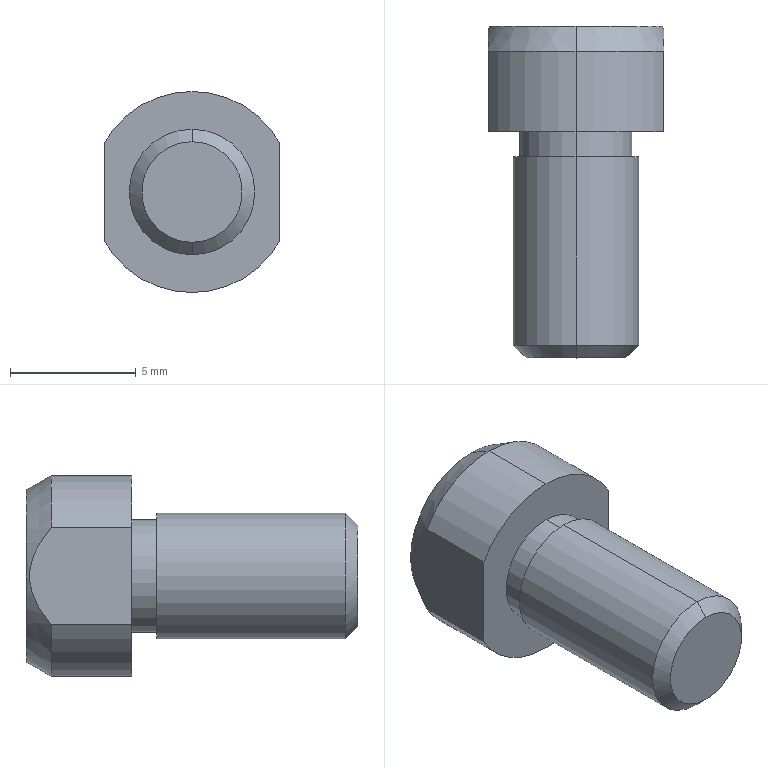Part | STEP file | PN_0011 Default | 1 solid | 17 faces | box 7 x 13.2 x 8 mm | volume 366.094 mm3 | cylinder 7 | plane 6 | cone 4 | commonest cylinder face diameters 8 x3 4.5 x2 5 x2
STEP:
#1=CARTESIAN_POINT('',(0.,14.722,-2.));
#2=VERTEX_POINT('',#1);
#3=CARTESIAN_POINT('',(0.,14.722,2.));
#4=VERTEX_POINT('',#3);
#5=CARTESIAN_POINT('',(0.,14.722,0.));
#6=DIRECTION('',(0.,-1.,0.));
#7=DIRECTION('',(0.,0.,-1.));
#8=AXIS2_PLACEMENT_3D('',#5,#6,#7);
#9=CIRCLE('',#8,2.);
#10=EDGE_CURVE('',#2,#4,#9,.T.);
#11=ORIENTED_EDGE('',*,*,#10,.F.);
#12=CARTESIAN_POINT('',(0.,15.222,-2.5));
#13=VERTEX_POINT('',#12);
#14=CARTESIAN_POINT('',(0.,15.222,-2.5));
#15=DIRECTION('',(0.,0.7071,-0.7071));
#16=VECTOR('',#15,1000.);
#17=LINE('',#14,#16);
#18=EDGE_CURVE('',#2,#13,#17,.T.);
#19=ORIENTED_EDGE('',*,*,#18,.T.);
#20=CARTESIAN_POINT('',(0.,15.222,2.5));
#21=VERTEX_POINT('',#20);
#22=CARTESIAN_POINT('',(0.,15.222,0.));
#23=DIRECTION('',(0.,1.,0.));
#24=DIRECTION('',(0.,0.,-1.));
#25=AXIS2_PLACEMENT_3D('',#22,#23,#24);
#26=CIRCLE('',#25,2.5);
#27=EDGE_CURVE('',#21,#13,#26,.T.);
#28=ORIENTED_EDGE('',*,*,#27,.F.);
#29=CARTESIAN_POINT('',(0.,15.222,2.5));
#30=DIRECTION('',(0.,0.7071,0.7071));
#31=VECTOR('',#30,1000.);
#32=LINE('',#29,#31);
#33=EDGE_CURVE('',#4,#21,#32,.T.);
#34=ORIENTED_EDGE('',*,*,#33,.F.);
#35=EDGE_LOOP('',(#11,#19,#28,#34));
#36=FACE_OUTER_BOUND('',#35,.T.);
#37=CARTESIAN_POINT('',(0.,15.222,0.));
#38=DIRECTION('',(0.,1.,0.));
#39=DIRECTION('',(0.,0.,1.));
#40=AXIS2_PLACEMENT_3D('',#37,#38,#39);
#41=CONICAL_SURFACE('',#40,2.5,0.7854);
#42=ADVANCED_FACE('',(#36),#41,.T.);
#43=ORIENTED_EDGE('',*,*,#27,.T.);
#44=CARTESIAN_POINT('',(0.,22.722,-2.5));
#45=VERTEX_POINT('',#44);
#46=CARTESIAN_POINT('',(0.,25.949,-2.5));
#47=DIRECTION('',(0.,1.,0.));
#48=VECTOR('',#47,1000.);
#49=LINE('',#46,#48);
#50=EDGE_CURVE('',#13,#45,#49,.T.);
#51=ORIENTED_EDGE('',*,*,#50,.T.);
#52=CARTESIAN_POINT('',(0.,22.722,2.5));
#53=VERTEX_POINT('',#52);
#54=CARTESIAN_POINT('',(0.,22.722,0.));
#55=DIRECTION('',(0.,1.,0.));
#56=DIRECTION('',(0.,0.,-1.));
#57=AXIS2_PLACEMENT_3D('',#54,#55,#56);
#58=CIRCLE('',#57,2.5);
#59=EDGE_CURVE('',#53,#45,#58,.T.);
#60=ORIENTED_EDGE('',*,*,#59,.F.);
#61=CARTESIAN_POINT('',(0.,25.949,2.5));
#62=DIRECTION('',(0.,1.,0.));
#63=VECTOR('',#62,1000.);
#64=LINE('',#61,#63);
#65=EDGE_CURVE('',#21,#53,#64,.T.);
#66=ORIENTED_EDGE('',*,*,#65,.F.);
#67=EDGE_LOOP('',(#43,#51,#60,#66));
#68=FACE_OUTER_BOUND('',#67,.T.);
#69=CARTESIAN_POINT('',(0.,25.949,0.));
#70=DIRECTION('',(0.,1.,0.));
#71=DIRECTION('',(0.,0.,1.));
#72=AXIS2_PLACEMENT_3D('',#69,#70,#71);
#73=CYLINDRICAL_SURFACE('',#72,2.5);
#74=ADVANCED_FACE('',(#68),#73,.T.);
#75=CARTESIAN_POINT('',(0.,22.722,-2.25));
#76=VERTEX_POINT('',#75);
#77=CARTESIAN_POINT('',(0.,22.722,2.25));
#78=VERTEX_POINT('',#77);
#79=CARTESIAN_POINT('',(0.,22.722,0.));
#80=DIRECTION('',(0.,-1.,0.));
#81=DIRECTION('',(0.,0.,-1.));
#82=AXIS2_PLACEMENT_3D('',#79,#80,#81);
#83=CIRCLE('',#82,2.25);
#84=EDGE_CURVE('',#76,#78,#83,.T.);
#85=ORIENTED_EDGE('',*,*,#84,.F.);
#86=CARTESIAN_POINT('',(0.,23.722,-2.25));
#87=VERTEX_POINT('',#86);
#88=CARTESIAN_POINT('',(0.,22.722,-2.25));
#89=DIRECTION('',(0.,1.,0.));
#90=VECTOR('',#89,1000.);
#91=LINE('',#88,#90);
#92=EDGE_CURVE('',#76,#87,#91,.T.);
#93=ORIENTED_EDGE('',*,*,#92,.T.);
#94=CARTESIAN_POINT('',(0.,23.722,2.25));
#95=VERTEX_POINT('',#94);
#96=CARTESIAN_POINT('',(0.,23.722,0.));
#97=DIRECTION('',(0.,-1.,0.));
#98=DIRECTION('',(0.,0.,-1.));
#99=AXIS2_PLACEMENT_3D('',#96,#97,#98);
#100=CIRCLE('',#99,2.25);
#101=EDGE_CURVE('',#87,#95,#100,.T.);
#102=ORIENTED_EDGE('',*,*,#101,.T.);
#103=CARTESIAN_POINT('',(0.,22.722,2.25));
#104=DIRECTION('',(0.,1.,0.));
#105=VECTOR('',#104,1000.);
#106=LINE('',#103,#105);
#107=EDGE_CURVE('',#78,#95,#106,.T.);
#108=ORIENTED_EDGE('',*,*,#107,.F.);
#109=EDGE_LOOP('',(#85,#93,#102,#108));
#110=FACE_OUTER_BOUND('',#109,.T.);
#111=CARTESIAN_POINT('',(0.,22.722,0.));
#112=DIRECTION('',(0.,1.,0.));
#113=DIRECTION('',(0.,0.,1.));
#114=AXIS2_PLACEMENT_3D('',#111,#112,#113);
#115=CYLINDRICAL_SURFACE('',#114,2.25);
#116=ADVANCED_FACE('',(#110),#115,.T.);
#117=CARTESIAN_POINT('',(0.,27.922,3.423));
#118=VERTEX_POINT('',#117);
#119=CARTESIAN_POINT('',(0.,27.922,-3.423));
#120=VERTEX_POINT('',#119);
#121=CARTESIAN_POINT('',(0.,27.922,0.));
#122=DIRECTION('',(0.,1.,0.));
#123=DIRECTION('',(0.,0.,1.));
#124=AXIS2_PLACEMENT_3D('',#121,#122,#123);
#125=CIRCLE('',#124,3.423);
#126=EDGE_CURVE('',#118,#120,#125,.T.);
#127=ORIENTED_EDGE('',*,*,#126,.F.);
#128=CARTESIAN_POINT('',(0.,26.922,4.));
#129=VERTEX_POINT('',#128);
#130=CARTESIAN_POINT('',(0.,27.922,3.423));
#131=DIRECTION('',(0.,-0.866,0.5));
#132=VECTOR('',#131,1000.);
#133=LINE('',#130,#132);
#134=EDGE_CURVE('',#118,#129,#133,.T.);
#135=ORIENTED_EDGE('',*,*,#134,.T.);
#136=CARTESIAN_POINT('',(3.5,26.922,1.936));
#137=VERTEX_POINT('',#136);
#138=CARTESIAN_POINT('',(0.,26.922,0.));
#139=DIRECTION('',(0.,-1.,0.));
#140=DIRECTION('',(0.,0.,1.));
#141=AXIS2_PLACEMENT_3D('',#138,#139,#140);
#142=CIRCLE('',#141,4.);
#143=EDGE_CURVE('',#137,#129,#142,.T.);
#144=ORIENTED_EDGE('',*,*,#143,.F.);
#145=CARTESIAN_POINT('',(3.5,26.922,-1.936));
#146=VERTEX_POINT('',#145);
#147=CARTESIAN_POINT('',(3.5,26.922,-1.936));
#148=CARTESIAN_POINT('',(3.5,27.153,-1.661));
#149=CARTESIAN_POINT('',(3.5,27.366,-1.364));
#150=CARTESIAN_POINT('',(3.5,27.608,-0.8747));
#151=CARTESIAN_POINT('',(3.5,27.673,-0.7067));
#152=CARTESIAN_POINT('',(3.5,27.764,-0.3574));
#153=CARTESIAN_POINT('',(3.5,27.789,-0.1747));
#154=CARTESIAN_POINT('',(3.5,27.788,0.184));
#155=CARTESIAN_POINT('',(3.5,27.763,0.364));
#156=CARTESIAN_POINT('',(3.5,27.67,0.7151));
#157=CARTESIAN_POINT('',(3.5,27.604,0.8824));
#158=CARTESIAN_POINT('',(3.5,27.444,1.205));
#159=CARTESIAN_POINT('',(3.5,27.35,1.361));
#160=CARTESIAN_POINT('',(3.5,27.146,1.658));
#161=CARTESIAN_POINT('',(3.5,27.037,1.8));
#162=CARTESIAN_POINT('',(3.5,26.922,1.936));
#163=B_SPLINE_CURVE_WITH_KNOTS('',3,(#147,#148,#149,#150,#151,#152,#153,#154,#155,#156,#157,#158,#159,#160,#161,#162),.UNSPECIFIED.,.F.,.F.,(4,2,2,2,2,2,2,4),(0.007144,0.008222,0.008761,0.0093,0.009839,0.01038,0.01092,0.01146),.UNSPECIFIED.);
#164=EDGE_CURVE('',#146,#137,#163,.T.);
#165=ORIENTED_EDGE('',*,*,#164,.F.);
#166=CARTESIAN_POINT('',(0.,26.922,-4.));
#167=VERTEX_POINT('',#166);
#168=CARTESIAN_POINT('',(0.,26.922,0.));
#169=DIRECTION('',(0.,-1.,0.));
#170=DIRECTION('',(0.,0.,1.));
#171=AXIS2_PLACEMENT_3D('',#168,#169,#170);
#172=CIRCLE('',#171,4.);
#173=EDGE_CURVE('',#167,#146,#172,.T.);
#174=ORIENTED_EDGE('',*,*,#173,.F.);
#175=CARTESIAN_POINT('',(0.,27.922,-3.423));
#176=DIRECTION('',(0.,-0.866,-0.5));
#177=VECTOR('',#176,1000.);
#178=LINE('',#175,#177);
#179=EDGE_CURVE('',#120,#167,#178,.T.);
#180=ORIENTED_EDGE('',*,*,#179,.F.);
#181=EDGE_LOOP('',(#127,#135,#144,#165,#174,#180));
#182=FACE_OUTER_BOUND('',#181,.T.);
#183=CARTESIAN_POINT('',(0.,27.922,0.));
#184=DIRECTION('',(0.,-1.,0.));
#185=DIRECTION('',(0.,0.,-1.));
#186=AXIS2_PLACEMENT_3D('',#183,#184,#185);
#187=CONICAL_SURFACE('',#186,3.423,0.5236);
#188=ADVANCED_FACE('',(#182),#187,.T.);
#189=CARTESIAN_POINT('',(-3.5,23.722,1.936));
#190=VERTEX_POINT('',#189);
#191=CARTESIAN_POINT('',(0.,23.722,4.));
#192=VERTEX_POINT('',#191);
#193=CARTESIAN_POINT('',(0.,23.722,0.));
#194=DIRECTION('',(0.,1.,0.));
#195=DIRECTION('',(0.,0.,1.));
#196=AXIS2_PLACEMENT_3D('',#193,#194,#195);
#197=CIRCLE('',#196,4.);
#198=EDGE_CURVE('',#190,#192,#197,.T.);
#199=ORIENTED_EDGE('',*,*,#198,.T.);
#200=CARTESIAN_POINT('',(0.,25.949,4.));
#201=DIRECTION('',(0.,1.,0.));
#202=VECTOR('',#201,1000.);
#203=LINE('',#200,#202);
#204=EDGE_CURVE('',#192,#129,#203,.T.);
#205=ORIENTED_EDGE('',*,*,#204,.T.);
#206=CARTESIAN_POINT('',(-3.5,26.922,1.936));
#207=VERTEX_POINT('',#206);
#208=CARTESIAN_POINT('',(0.,26.922,0.));
#209=DIRECTION('',(0.,-1.,0.));
#210=DIRECTION('',(0.,0.,1.));
#211=AXIS2_PLACEMENT_3D('',#208,#209,#210);
#212=CIRCLE('',#211,4.);
#213=EDGE_CURVE('',#129,#207,#212,.T.);
#214=ORIENTED_EDGE('',*,*,#213,.T.);
#215=CARTESIAN_POINT('',(-3.5,25.949,1.936));
#216=DIRECTION('',(0.,1.,0.));
#217=VECTOR('',#216,1000.);
#218=LINE('',#215,#217);
#219=EDGE_CURVE('',#190,#207,#218,.T.);
#220=ORIENTED_EDGE('',*,*,#219,.F.);
#221=EDGE_LOOP('',(#199,#205,#214,#220));
#222=FACE_OUTER_BOUND('',#221,.T.);
#223=CARTESIAN_POINT('',(0.,25.949,0.));
#224=DIRECTION('',(0.,1.,0.));
#225=DIRECTION('',(0.,0.,1.));
#226=AXIS2_PLACEMENT_3D('',#223,#224,#225);
#227=CYLINDRICAL_SURFACE('',#226,4.);
#228=ADVANCED_FACE('',(#222),#227,.T.);
#229=ORIENTED_EDGE('',*,*,#204,.F.);
#230=CARTESIAN_POINT('',(3.5,23.722,1.936));
#231=VERTEX_POINT('',#230);
#232=CARTESIAN_POINT('',(0.,23.722,0.));
#233=DIRECTION('',(0.,1.,0.));
#234=DIRECTION('',(0.,0.,1.));
#235=AXIS2_PLACEMENT_3D('',#232,#233,#234);
#236=CIRCLE('',#235,4.);
#237=EDGE_CURVE('',#192,#231,#236,.T.);
#238=ORIENTED_EDGE('',*,*,#237,.T.);
#239=CARTESIAN_POINT('',(3.5,25.949,1.936));
#240=DIRECTION('',(0.,-1.,0.));
#241=VECTOR('',#240,1000.);
#242=LINE('',#239,#241);
#243=EDGE_CURVE('',#137,#231,#242,.T.);
#244=ORIENTED_EDGE('',*,*,#243,.F.);
#245=ORIENTED_EDGE('',*,*,#143,.T.);
#246=EDGE_LOOP('',(#229,#238,#244,#245));
#247=FACE_OUTER_BOUND('',#246,.T.);
#248=CARTESIAN_POINT('',(0.,25.949,0.));
#249=DIRECTION('',(0.,1.,0.));
#250=DIRECTION('',(0.,0.,1.));
#251=AXIS2_PLACEMENT_3D('',#248,#249,#250);
#252=CYLINDRICAL_SURFACE('',#251,4.);
#253=ADVANCED_FACE('',(#247),#252,.T.);
#254=CARTESIAN_POINT('',(0.,27.922,0.));
#255=DIRECTION('',(0.,1.,0.));
#256=DIRECTION('',(0.,0.,1.));
#257=AXIS2_PLACEMENT_3D('',#254,#255,#256);
#258=CIRCLE('',#257,3.423);
#259=EDGE_CURVE('',#120,#118,#258,.T.);
#260=ORIENTED_EDGE('',*,*,#259,.T.);
#261=ORIENTED_EDGE('',*,*,#126,.T.);
#262=EDGE_LOOP('',(#260,#261));
#263=FACE_OUTER_BOUND('',#262,.T.);
#264=CARTESIAN_POINT('',(0.,27.922,0.));
#265=DIRECTION('',(0.,1.,0.));
#266=DIRECTION('',(0.,0.,1.));
#267=AXIS2_PLACEMENT_3D('',#264,#265,#266);
#268=PLANE('',#267);
#269=ADVANCED_FACE('',(#263),#268,.T.);
#270=CARTESIAN_POINT('',(3.5,23.722,-1.936));
#271=VERTEX_POINT('',#270);
#272=CARTESIAN_POINT('',(3.5,25.949,-1.936));
#273=DIRECTION('',(0.,1.,0.));
#274=VECTOR('',#273,1000.);
#275=LINE('',#272,#274);
#276=EDGE_CURVE('',#271,#146,#275,.T.);
#277=ORIENTED_EDGE('',*,*,#276,.F.);
#278=CARTESIAN_POINT('',(-3.5,23.722,-1.936));
#279=VERTEX_POINT('',#278);
#280=CARTESIAN_POINT('',(0.,23.722,0.));
#281=DIRECTION('',(0.,1.,0.));
#282=DIRECTION('',(0.,0.,1.));
#283=AXIS2_PLACEMENT_3D('',#280,#281,#282);
#284=CIRCLE('',#283,4.);
#285=EDGE_CURVE('',#271,#279,#284,.T.);
#286=ORIENTED_EDGE('',*,*,#285,.T.);
#287=CARTESIAN_POINT('',(-3.5,26.922,-1.936));
#288=VERTEX_POINT('',#287);
#289=CARTESIAN_POINT('',(-3.5,25.949,-1.936));
#290=DIRECTION('',(0.,-1.,0.));
#291=VECTOR('',#290,1000.);
#292=LINE('',#289,#291);
#293=EDGE_CURVE('',#288,#279,#292,.T.);
#294=ORIENTED_EDGE('',*,*,#293,.F.);
#295=CARTESIAN_POINT('',(0.,26.922,0.));
#296=DIRECTION('',(0.,-1.,0.));
#297=DIRECTION('',(0.,0.,1.));
#298=AXIS2_PLACEMENT_3D('',#295,#296,#297);
#299=CIRCLE('',#298,4.);
#300=EDGE_CURVE('',#288,#167,#299,.T.);
#301=ORIENTED_EDGE('',*,*,#300,.T.);
#302=ORIENTED_EDGE('',*,*,#173,.T.);
#303=EDGE_LOOP('',(#277,#286,#294,#301,#302));
#304=FACE_OUTER_BOUND('',#303,.T.);
#305=CARTESIAN_POINT('',(0.,25.949,0.));
#306=DIRECTION('',(0.,1.,0.));
#307=DIRECTION('',(0.,0.,1.));
#308=AXIS2_PLACEMENT_3D('',#305,#306,#307);
#309=CYLINDRICAL_SURFACE('',#308,4.);
#310=ADVANCED_FACE('',(#304),#309,.T.);
#311=CARTESIAN_POINT('',(3.5,23.722,0.));
#312=DIRECTION('',(0.,0.,-1.));
#313=VECTOR('',#312,1000.);
#314=LINE('',#311,#313);
#315=EDGE_CURVE('',#231,#271,#314,.T.);
#316=ORIENTED_EDGE('',*,*,#315,.F.);
#317=ORIENTED_EDGE('',*,*,#237,.F.);
#318=ORIENTED_EDGE('',*,*,#198,.F.);
#319=CARTESIAN_POINT('',(-3.5,23.722,0.));
#320=DIRECTION('',(0.,0.,1.));
#321=VECTOR('',#320,1000.);
#322=LINE('',#319,#321);
#323=EDGE_CURVE('',#279,#190,#322,.T.);
#324=ORIENTED_EDGE('',*,*,#323,.F.);
#325=ORIENTED_EDGE('',*,*,#285,.F.);
#326=EDGE_LOOP('',(#316,#317,#318,#324,#325));
#327=FACE_OUTER_BOUND('',#326,.T.);
#328=CARTESIAN_POINT('',(0.,23.722,0.));
#329=DIRECTION('',(0.,-1.,0.));
#330=DIRECTION('',(0.,0.,-1.));
#331=AXIS2_PLACEMENT_3D('',#328,#329,#330);
#332=CIRCLE('',#331,2.25);
#333=EDGE_CURVE('',#95,#87,#332,.T.);
#334=ORIENTED_EDGE('',*,*,#333,.F.);
#335=ORIENTED_EDGE('',*,*,#101,.F.);
#336=EDGE_LOOP('',(#334,#335));
#337=FACE_BOUND('',#336,.T.);
#338=CARTESIAN_POINT('',(-4.,23.722,0.));
#339=DIRECTION('',(0.,-1.,0.));
#340=DIRECTION('',(0.,0.,-1.));
#341=AXIS2_PLACEMENT_3D('',#338,#339,#340);
#342=PLANE('',#341);
#343=ADVANCED_FACE('',(#327,#337),#342,.T.);
#344=ORIENTED_EDGE('',*,*,#134,.F.);
#345=ORIENTED_EDGE('',*,*,#259,.F.);
#346=ORIENTED_EDGE('',*,*,#179,.T.);
#347=ORIENTED_EDGE('',*,*,#300,.F.);
#348=CARTESIAN_POINT('',(-3.5,26.922,1.936));
#349=CARTESIAN_POINT('',(-3.5,27.037,1.8));
#350=CARTESIAN_POINT('',(-3.5,27.146,1.658));
#351=CARTESIAN_POINT('',(-3.5,27.35,1.361));
#352=CARTESIAN_POINT('',(-3.5,27.444,1.205));
#353=CARTESIAN_POINT('',(-3.5,27.604,0.8824));
#354=CARTESIAN_POINT('',(-3.5,27.67,0.7151));
#355=CARTESIAN_POINT('',(-3.5,27.763,0.364));
#356=CARTESIAN_POINT('',(-3.5,27.788,0.184));
#357=CARTESIAN_POINT('',(-3.5,27.789,-0.1747));
#358=CARTESIAN_POINT('',(-3.5,27.764,-0.3574));
#359=CARTESIAN_POINT('',(-3.5,27.673,-0.7067));
#360=CARTESIAN_POINT('',(-3.5,27.608,-0.8747));
#361=CARTESIAN_POINT('',(-3.5,27.366,-1.364));
#362=CARTESIAN_POINT('',(-3.5,27.153,-1.661));
#363=CARTESIAN_POINT('',(-3.5,26.922,-1.936));
#364=B_SPLINE_CURVE_WITH_KNOTS('',3,(#348,#349,#350,#351,#352,#353,#354,#355,#356,#357,#358,#359,#360,#361,#362,#363),.UNSPECIFIED.,.F.,.F.,(4,2,2,2,2,2,2,4),(0.001496,0.002031,0.002567,0.003102,0.003638,0.004173,0.004709,0.00578),.UNSPECIFIED.);
#365=EDGE_CURVE('',#207,#288,#364,.T.);
#366=ORIENTED_EDGE('',*,*,#365,.F.);
#367=ORIENTED_EDGE('',*,*,#213,.F.);
#368=EDGE_LOOP('',(#344,#345,#346,#347,#366,#367));
#369=FACE_OUTER_BOUND('',#368,.T.);
#370=CARTESIAN_POINT('',(0.,27.922,0.));
#371=DIRECTION('',(0.,-1.,0.));
#372=DIRECTION('',(0.,0.,-1.));
#373=AXIS2_PLACEMENT_3D('',#370,#371,#372);
#374=CONICAL_SURFACE('',#373,3.423,0.5236);
#375=ADVANCED_FACE('',(#369),#374,.T.);
#376=ORIENTED_EDGE('',*,*,#59,.T.);
#377=CARTESIAN_POINT('',(0.,22.722,0.));
#378=DIRECTION('',(0.,1.,0.));
#379=DIRECTION('',(0.,0.,-1.));
#380=AXIS2_PLACEMENT_3D('',#377,#378,#379);
#381=CIRCLE('',#380,2.5);
#382=EDGE_CURVE('',#45,#53,#381,.T.);
#383=ORIENTED_EDGE('',*,*,#382,.T.);
#384=EDGE_LOOP('',(#376,#383));
#385=FACE_OUTER_BOUND('',#384,.T.);
#386=CARTESIAN_POINT('',(0.,22.722,0.));
#387=DIRECTION('',(0.,-1.,0.));
#388=DIRECTION('',(0.,0.,-1.));
#389=AXIS2_PLACEMENT_3D('',#386,#387,#388);
#390=CIRCLE('',#389,2.25);
#391=EDGE_CURVE('',#78,#76,#390,.T.);
#392=ORIENTED_EDGE('',*,*,#391,.T.);
#393=ORIENTED_EDGE('',*,*,#84,.T.);
#394=EDGE_LOOP('',(#392,#393));
#395=FACE_BOUND('',#394,.T.);
#396=CARTESIAN_POINT('',(0.,22.722,0.));
#397=DIRECTION('',(0.,-1.,0.));
#398=DIRECTION('',(0.,0.,-1.));
#399=AXIS2_PLACEMENT_3D('',#396,#397,#398);
#400=PLANE('',#399);
#401=ADVANCED_FACE('',(#385,#395),#400,.F.);
#402=ORIENTED_EDGE('',*,*,#92,.F.);
#403=ORIENTED_EDGE('',*,*,#391,.F.);
#404=ORIENTED_EDGE('',*,*,#107,.T.);
#405=ORIENTED_EDGE('',*,*,#333,.T.);
#406=EDGE_LOOP('',(#402,#403,#404,#405));
#407=FACE_OUTER_BOUND('',#406,.T.);
#408=CARTESIAN_POINT('',(0.,22.722,0.));
#409=DIRECTION('',(0.,1.,0.));
#410=DIRECTION('',(0.,0.,1.));
#411=AXIS2_PLACEMENT_3D('',#408,#409,#410);
#412=CYLINDRICAL_SURFACE('',#411,2.25);
#413=ADVANCED_FACE('',(#407),#412,.T.);
#414=CARTESIAN_POINT('',(0.,14.722,0.));
#415=DIRECTION('',(0.,-1.,0.));
#416=DIRECTION('',(0.,0.,-1.));
#417=AXIS2_PLACEMENT_3D('',#414,#415,#416);
#418=CIRCLE('',#417,2.);
#419=EDGE_CURVE('',#4,#2,#418,.T.);
#420=ORIENTED_EDGE('',*,*,#419,.T.);
#421=ORIENTED_EDGE('',*,*,#10,.T.);
#422=EDGE_LOOP('',(#420,#421));
#423=FACE_OUTER_BOUND('',#422,.T.);
#424=CARTESIAN_POINT('',(-2.5,14.722,0.));
#425=DIRECTION('',(0.,-1.,0.));
#426=DIRECTION('',(0.,0.,-1.));
#427=AXIS2_PLACEMENT_3D('',#424,#425,#426);
#428=PLANE('',#427);
#429=ADVANCED_FACE('',(#423),#428,.T.);
#430=ORIENTED_EDGE('',*,*,#50,.F.);
#431=CARTESIAN_POINT('',(0.,15.222,0.));
#432=DIRECTION('',(0.,1.,0.));
#433=DIRECTION('',(0.,0.,-1.));
#434=AXIS2_PLACEMENT_3D('',#431,#432,#433);
#435=CIRCLE('',#434,2.5);
#436=EDGE_CURVE('',#13,#21,#435,.T.);
#437=ORIENTED_EDGE('',*,*,#436,.T.);
#438=ORIENTED_EDGE('',*,*,#65,.T.);
#439=ORIENTED_EDGE('',*,*,#382,.F.);
#440=EDGE_LOOP('',(#430,#437,#438,#439));
#441=FACE_OUTER_BOUND('',#440,.T.);
#442=CARTESIAN_POINT('',(0.,25.949,0.));
#443=DIRECTION('',(0.,1.,0.));
#444=DIRECTION('',(0.,0.,1.));
#445=AXIS2_PLACEMENT_3D('',#442,#443,#444);
#446=CYLINDRICAL_SURFACE('',#445,2.5);
#447=ADVANCED_FACE('',(#441),#446,.T.);
#448=ORIENTED_EDGE('',*,*,#18,.F.);
#449=ORIENTED_EDGE('',*,*,#419,.F.);
#450=ORIENTED_EDGE('',*,*,#33,.T.);
#451=ORIENTED_EDGE('',*,*,#436,.F.);
#452=EDGE_LOOP('',(#448,#449,#450,#451));
#453=FACE_OUTER_BOUND('',#452,.T.);
#454=CARTESIAN_POINT('',(0.,15.222,0.));
#455=DIRECTION('',(0.,1.,0.));
#456=DIRECTION('',(0.,0.,1.));
#457=AXIS2_PLACEMENT_3D('',#454,#455,#456);
#458=CONICAL_SURFACE('',#457,2.5,0.7854);
#459=ADVANCED_FACE('',(#453),#458,.T.);
#460=ORIENTED_EDGE('',*,*,#323,.T.);
#461=ORIENTED_EDGE('',*,*,#219,.T.);
#462=ORIENTED_EDGE('',*,*,#365,.T.);
#463=ORIENTED_EDGE('',*,*,#293,.T.);
#464=EDGE_LOOP('',(#460,#461,#462,#463));
#465=FACE_OUTER_BOUND('',#464,.T.);
#466=CARTESIAN_POINT('',(-3.5,17.922,-4.03));
#467=DIRECTION('',(1.,0.,0.));
#468=DIRECTION('',(0.,0.,-1.));
#469=AXIS2_PLACEMENT_3D('',#466,#467,#468);
#470=PLANE('',#469);
#471=ADVANCED_FACE('',(#465),#470,.F.);
#472=ORIENTED_EDGE('',*,*,#315,.T.);
#473=ORIENTED_EDGE('',*,*,#276,.T.);
#474=ORIENTED_EDGE('',*,*,#164,.T.);
#475=ORIENTED_EDGE('',*,*,#243,.T.);
#476=EDGE_LOOP('',(#472,#473,#474,#475));
#477=FACE_OUTER_BOUND('',#476,.T.);
#478=CARTESIAN_POINT('',(3.5,17.922,-4.03));
#479=DIRECTION('',(-1.,0.,0.));
#480=DIRECTION('',(0.,0.,1.));
#481=AXIS2_PLACEMENT_3D('',#478,#479,#480);
#482=PLANE('',#481);
#483=ADVANCED_FACE('',(#477),#482,.F.);
#484=CLOSED_SHELL('',(#42,#74,#116,#188,#228,#253,#269,#310,#343,#375,#401,#413,#429,#447,#459,#471,#483));
#485=MANIFOLD_SOLID_BREP('',#484);
#486=CARTESIAN_POINT('',(0.,0.,0.));
#487=DIRECTION('',(0.,0.,1.));
#488=DIRECTION('',(1.,0.,0.));
#489=AXIS2_PLACEMENT_3D('',#486,#487,#488);
#490=(LENGTH_UNIT()NAMED_UNIT(*)SI_UNIT(.MILLI.,.METRE.));
#491=UNCERTAINTY_MEASURE_WITH_UNIT(LENGTH_MEASURE(0.00001),#490,'','');
#492=(NAMED_UNIT(*)PLANE_ANGLE_UNIT()SI_UNIT($,.RADIAN.));
#493=(NAMED_UNIT(*)SI_UNIT($,.STERADIAN.)SOLID_ANGLE_UNIT());
#494=(GEOMETRIC_REPRESENTATION_CONTEXT(3)GLOBAL_UNCERTAINTY_ASSIGNED_CONTEXT((#491))GLOBAL_UNIT_ASSIGNED_CONTEXT((#490,#492,#493))REPRESENTATION_CONTEXT('',''));
#495=ADVANCED_BREP_SHAPE_REPRESENTATION('',(#485,#489),#494);